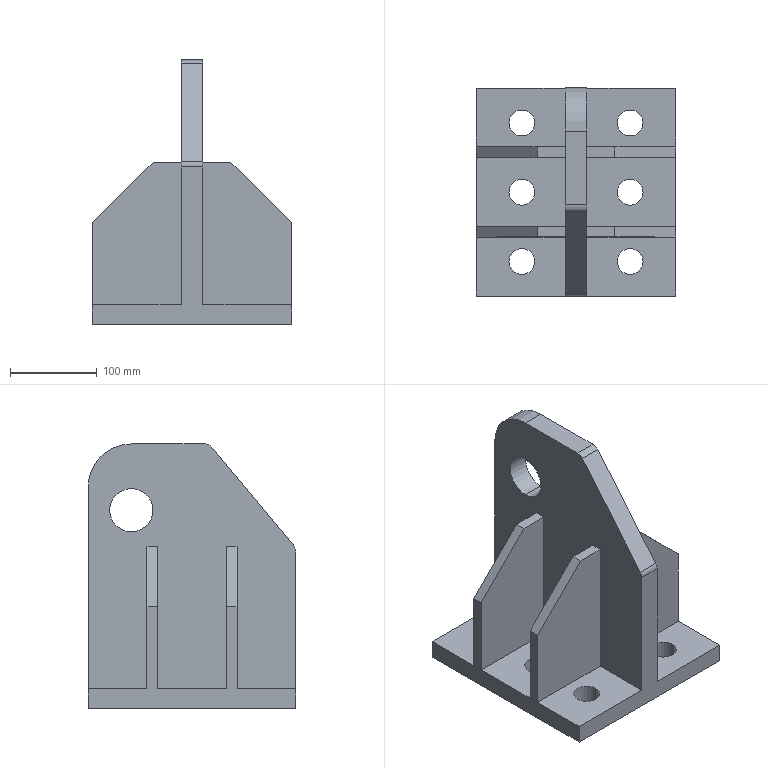Part | STEP file | SX-lifting lug | 1 solid | 48 faces | box 230 x 240 x 305 mm | volume 3300682 mm3 | plane 31 | cylinder 17 | commonest cylinder face diameters 30 x12 20 x2 50 x2 100 x1